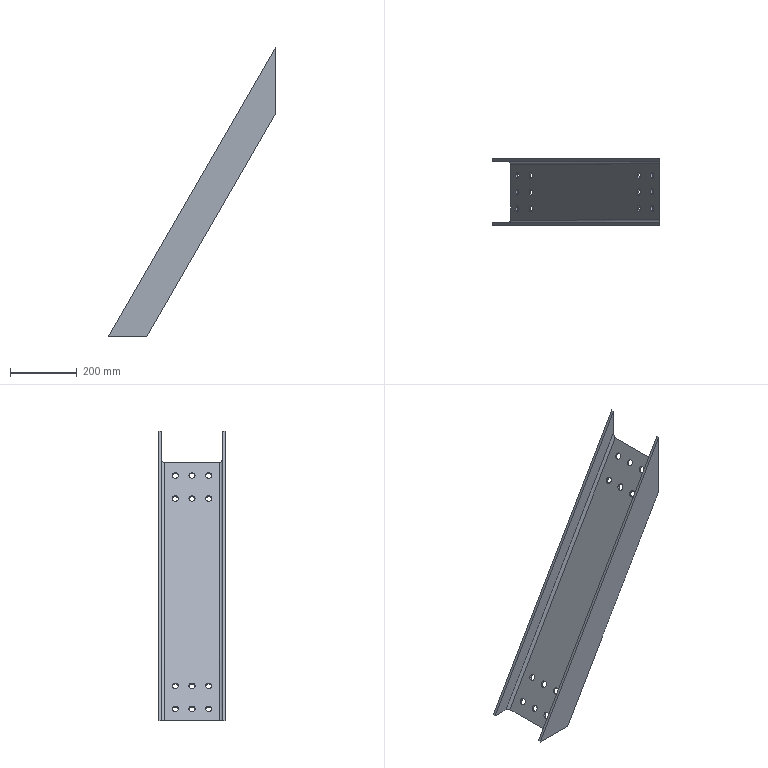Part | STEP file | Powder bin diagonal beam 1_Default<As Machined> | 1 solid | 42 faces | box 502.735 x 200 x 870.763 mm | volume 2354862 mm3 | cylinder 28 | plane 14 | commonest cylinder face diameters 19 x24 16 x4